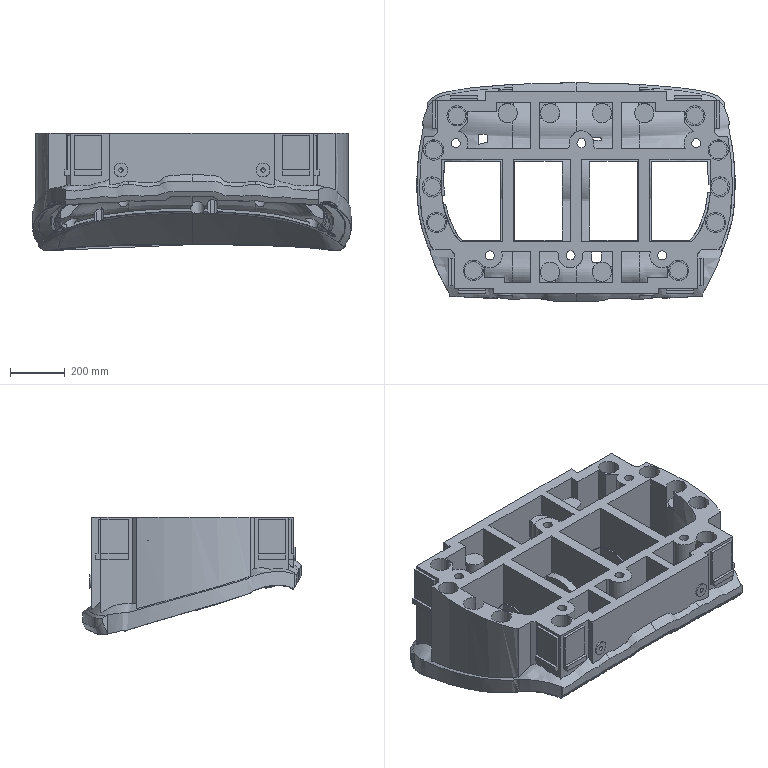Part | NX | features solid 2 | 1 solid | 1234 faces | box 1164 x 798.168 x 431.102 mm | volume 71968323 mm3 | spline 907 | plane 238 | cylinder 81 | cone 8 | commonest cylinder face diameters 20 x21 50 x14 74 x10 16 x8 64 x7 33 x6